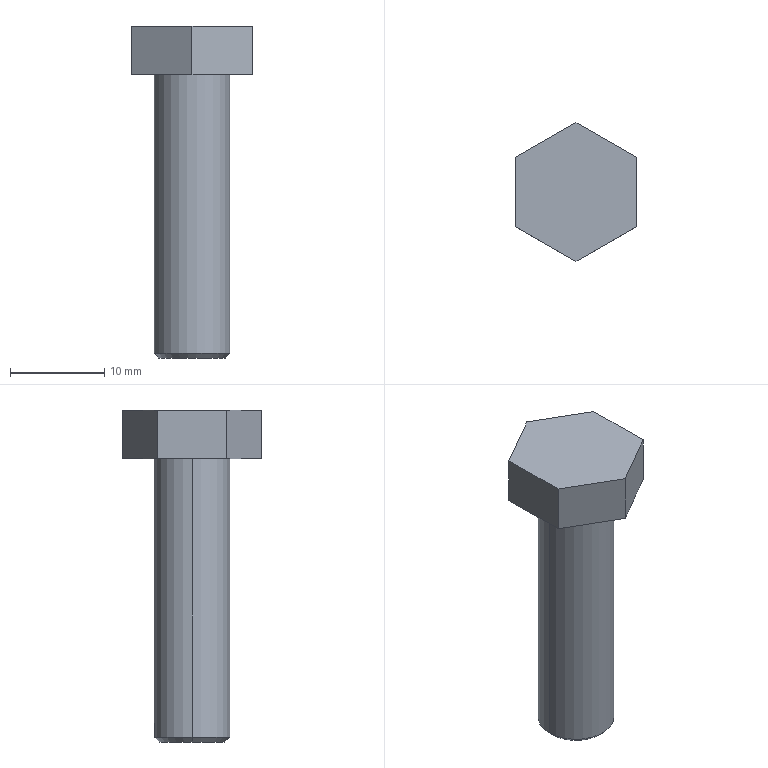Part | STEP file | Bulong M8_3F | 1 solid | 13 faces | box 12.73 x 14.699 x 35.15 mm | volume 2228 mm3 | plane 9 | cone 2 | cylinder 2 | commonest cylinder face diameters 8 x2
STEP:
#1=CARTESIAN_POINT('',(0.,0.,0.));
#2=DIRECTION('',(0.,0.,1.));
#3=DIRECTION('',(1.,0.,0.));
#4=AXIS2_PLACEMENT_3D('',#1,#2,#3);
#5=CARTESIAN_POINT('',(-3.5,0.,-30.));
#6=VERTEX_POINT('',#5);
#7=CARTESIAN_POINT('',(3.5,0.,-30.));
#8=VERTEX_POINT('',#7);
#9=CARTESIAN_POINT('',(0.,0.,-30.));
#10=DIRECTION('',(0.,0.,-1.));
#11=DIRECTION('',(-1.,0.,0.));
#12=AXIS2_PLACEMENT_3D('',#9,#10,#11);
#13=CIRCLE('',#12,3.5);
#14=CARTESIAN_POINT('',(0.,0.,-30.));
#15=DIRECTION('',(0.,0.,1.));
#16=DIRECTION('',(1.,0.,0.));
#17=AXIS2_PLACEMENT_3D('',#14,#15,#16);
#18=CONICAL_SURFACE('',#17,3.5,0.7854);
#19=CARTESIAN_POINT('',(3.142,0.));
#20=DIRECTION('',(-1.,0.));
#21=VECTOR('',#20,1.);
#22=LINE('',#19,#21);
#23=(GEOMETRIC_REPRESENTATION_CONTEXT(2)PARAMETRIC_REPRESENTATION_CONTEXT()REPRESENTATION_CONTEXT('',''));
#24=DEFINITIONAL_REPRESENTATION('',(#22),#23);
#25=PCURVE('',#18,#24);
#26=CARTESIAN_POINT('',(0.,0.,-30.));
#27=DIRECTION('',(0.,0.,-1.));
#28=DIRECTION('',(-1.,0.,0.));
#29=AXIS2_PLACEMENT_3D('',#26,#27,#28);
#30=PLANE('',#29);
#31=CARTESIAN_POINT('',(0.,0.));
#32=DIRECTION('',(1.,0.));
#33=AXIS2_PLACEMENT_2D('',#31,#32);
#34=CIRCLE('',#33,3.5);
#35=(GEOMETRIC_REPRESENTATION_CONTEXT(2)PARAMETRIC_REPRESENTATION_CONTEXT()REPRESENTATION_CONTEXT('',''));
#36=DEFINITIONAL_REPRESENTATION('',(#34),#35);
#37=PCURVE('',#30,#36);
#38=SURFACE_CURVE('',#13,(#25,#37),.PCURVE_S1.);
#39=EDGE_CURVE('',#6,#8,#38,.T.);
#40=ORIENTED_EDGE('',*,*,#39,.F.);
#41=CARTESIAN_POINT('',(-4.,0.,-29.5));
#42=VERTEX_POINT('',#41);
#43=CARTESIAN_POINT('',(-3.5,0.,-30.));
#44=DIRECTION('',(-0.7071,0.,0.7071));
#45=VECTOR('',#44,1.);
#46=LINE('',#43,#45);
#47=CARTESIAN_POINT('',(3.142,0.));
#48=DIRECTION('',(0.,1.));
#49=VECTOR('',#48,1.);
#50=LINE('',#47,#49);
#51=(GEOMETRIC_REPRESENTATION_CONTEXT(2)PARAMETRIC_REPRESENTATION_CONTEXT()REPRESENTATION_CONTEXT('',''));
#52=DEFINITIONAL_REPRESENTATION('',(#50),#51);
#53=PCURVE('',#18,#52);
#54=CARTESIAN_POINT('',(0.,0.,-30.));
#55=DIRECTION('',(0.,0.,1.));
#56=DIRECTION('',(1.,0.,0.));
#57=AXIS2_PLACEMENT_3D('',#54,#55,#56);
#58=CONICAL_SURFACE('',#57,3.5,0.7854);
#59=CARTESIAN_POINT('',(3.142,0.));
#60=DIRECTION('',(0.,1.));
#61=VECTOR('',#60,1.);
#62=LINE('',#59,#61);
#63=(GEOMETRIC_REPRESENTATION_CONTEXT(2)PARAMETRIC_REPRESENTATION_CONTEXT()REPRESENTATION_CONTEXT('',''));
#64=DEFINITIONAL_REPRESENTATION('',(#62),#63);
#65=PCURVE('',#58,#64);
#66=SURFACE_CURVE('',#46,(#53,#65),.PCURVE_S1.);
#67=EDGE_CURVE('',#6,#42,#66,.T.);
#68=ORIENTED_EDGE('',*,*,#67,.T.);
#69=CARTESIAN_POINT('',(4.,0.,-29.5));
#70=VERTEX_POINT('',#69);
#71=CARTESIAN_POINT('',(0.,0.,-29.5));
#72=DIRECTION('',(0.,0.,1.));
#73=DIRECTION('',(-1.,0.,0.));
#74=AXIS2_PLACEMENT_3D('',#71,#72,#73);
#75=CIRCLE('',#74,4.);
#76=CARTESIAN_POINT('',(-3.142,0.5));
#77=DIRECTION('',(1.,0.));
#78=VECTOR('',#77,1.);
#79=LINE('',#76,#78);
#80=(GEOMETRIC_REPRESENTATION_CONTEXT(2)PARAMETRIC_REPRESENTATION_CONTEXT()REPRESENTATION_CONTEXT('',''));
#81=DEFINITIONAL_REPRESENTATION('',(#79),#80);
#82=PCURVE('',#18,#81);
#83=CARTESIAN_POINT('',(0.,0.,-30.));
#84=DIRECTION('',(0.,0.,1.));
#85=DIRECTION('',(1.,0.,0.));
#86=AXIS2_PLACEMENT_3D('',#83,#84,#85);
#87=CYLINDRICAL_SURFACE('',#86,4.);
#88=CARTESIAN_POINT('',(-3.142,0.5));
#89=DIRECTION('',(1.,0.));
#90=VECTOR('',#89,1.);
#91=LINE('',#88,#90);
#92=(GEOMETRIC_REPRESENTATION_CONTEXT(2)PARAMETRIC_REPRESENTATION_CONTEXT()REPRESENTATION_CONTEXT('',''));
#93=DEFINITIONAL_REPRESENTATION('',(#91),#92);
#94=PCURVE('',#87,#93);
#95=SURFACE_CURVE('',#75,(#82,#94),.PCURVE_S1.);
#96=EDGE_CURVE('',#70,#42,#95,.T.);
#97=ORIENTED_EDGE('',*,*,#96,.F.);
#98=CARTESIAN_POINT('',(3.5,0.,-30.));
#99=DIRECTION('',(0.7071,0.,0.7071));
#100=VECTOR('',#99,1.);
#101=LINE('',#98,#100);
#102=CARTESIAN_POINT('',(0.,0.));
#103=DIRECTION('',(0.,1.));
#104=VECTOR('',#103,1.);
#105=LINE('',#102,#104);
#106=(GEOMETRIC_REPRESENTATION_CONTEXT(2)PARAMETRIC_REPRESENTATION_CONTEXT()REPRESENTATION_CONTEXT('',''));
#107=DEFINITIONAL_REPRESENTATION('',(#105),#106);
#108=PCURVE('',#18,#107);
#109=CARTESIAN_POINT('',(6.283,0.));
#110=DIRECTION('',(0.,1.));
#111=VECTOR('',#110,1.);
#112=LINE('',#109,#111);
#113=(GEOMETRIC_REPRESENTATION_CONTEXT(2)PARAMETRIC_REPRESENTATION_CONTEXT()REPRESENTATION_CONTEXT('',''));
#114=DEFINITIONAL_REPRESENTATION('',(#112),#113);
#115=PCURVE('',#58,#114);
#116=SURFACE_CURVE('',#101,(#108,#115),.PCURVE_S1.);
#117=EDGE_CURVE('',#8,#70,#116,.T.);
#118=ORIENTED_EDGE('',*,*,#117,.F.);
#119=EDGE_LOOP('',(#40,#68,#97,#118));
#120=FACE_BOUND('',#119,.T.);
#121=ADVANCED_FACE('',(#120),#18,.T.);
#122=ORIENTED_EDGE('',*,*,#96,.T.);
#123=CARTESIAN_POINT('',(-4.,0.,0.));
#124=VERTEX_POINT('',#123);
#125=CARTESIAN_POINT('',(-4.,0.,-30.));
#126=DIRECTION('',(0.,0.,1.));
#127=VECTOR('',#126,1.);
#128=LINE('',#125,#127);
#129=CARTESIAN_POINT('',(3.142,0.));
#130=DIRECTION('',(0.,1.));
#131=VECTOR('',#130,1.);
#132=LINE('',#129,#131);
#133=(GEOMETRIC_REPRESENTATION_CONTEXT(2)PARAMETRIC_REPRESENTATION_CONTEXT()REPRESENTATION_CONTEXT('',''));
#134=DEFINITIONAL_REPRESENTATION('',(#132),#133);
#135=PCURVE('',#87,#134);
#136=CARTESIAN_POINT('',(0.,0.,-30.));
#137=DIRECTION('',(0.,0.,1.));
#138=DIRECTION('',(1.,0.,0.));
#139=AXIS2_PLACEMENT_3D('',#136,#137,#138);
#140=CYLINDRICAL_SURFACE('',#139,4.);
#141=CARTESIAN_POINT('',(3.142,0.));
#142=DIRECTION('',(0.,1.));
#143=VECTOR('',#142,1.);
#144=LINE('',#141,#143);
#145=(GEOMETRIC_REPRESENTATION_CONTEXT(2)PARAMETRIC_REPRESENTATION_CONTEXT()REPRESENTATION_CONTEXT('',''));
#146=DEFINITIONAL_REPRESENTATION('',(#144),#145);
#147=PCURVE('',#140,#146);
#148=SURFACE_CURVE('',#128,(#135,#147),.PCURVE_S1.);
#149=EDGE_CURVE('',#42,#124,#148,.T.);
#150=ORIENTED_EDGE('',*,*,#149,.T.);
#151=CARTESIAN_POINT('',(4.,0.,0.));
#152=VERTEX_POINT('',#151);
#153=CARTESIAN_POINT('',(0.,0.,0.));
#154=DIRECTION('',(0.,0.,-1.));
#155=DIRECTION('',(1.,0.,0.));
#156=AXIS2_PLACEMENT_3D('',#153,#154,#155);
#157=CIRCLE('',#156,4.);
#158=CARTESIAN_POINT('',(6.283,30.));
#159=DIRECTION('',(-1.,0.));
#160=VECTOR('',#159,1.);
#161=LINE('',#158,#160);
#162=(GEOMETRIC_REPRESENTATION_CONTEXT(2)PARAMETRIC_REPRESENTATION_CONTEXT()REPRESENTATION_CONTEXT('',''));
#163=DEFINITIONAL_REPRESENTATION('',(#161),#162);
#164=PCURVE('',#87,#163);
#165=CARTESIAN_POINT('',(0.,0.,0.));
#166=DIRECTION('',(0.,0.,1.));
#167=DIRECTION('',(1.,0.,0.));
#168=AXIS2_PLACEMENT_3D('',#165,#166,#167);
#169=PLANE('',#168);
#170=CARTESIAN_POINT('',(4.,0.));
#171=CARTESIAN_POINT('',(4.,-6.928));
#172=CARTESIAN_POINT('',(-2.,-3.464));
#173=CARTESIAN_POINT('',(-8.,0.));
#174=CARTESIAN_POINT('',(-2.,3.464));
#175=CARTESIAN_POINT('',(4.,6.928));
#176=CARTESIAN_POINT('',(4.,0.));
#177=(BOUNDED_CURVE()B_SPLINE_CURVE(2,(#170,#171,#172,#173,#174,#175,#176),.UNSPECIFIED.,.T.,.F.)B_SPLINE_CURVE_WITH_KNOTS((1,2,2,2,2,1),(-2.094,0.,2.094,4.189,6.283,8.378),.UNSPECIFIED.)CURVE()GEOMETRIC_REPRESENTATION_ITEM()RATIONAL_B_SPLINE_CURVE((1.,0.5,1.,0.5,1.,0.5,1.))REPRESENTATION_ITEM(''));
#178=(GEOMETRIC_REPRESENTATION_CONTEXT(2)PARAMETRIC_REPRESENTATION_CONTEXT()REPRESENTATION_CONTEXT('',''));
#179=DEFINITIONAL_REPRESENTATION('',(#177),#178);
#180=PCURVE('',#169,#179);
#181=SURFACE_CURVE('',#157,(#164,#180),.PCURVE_S1.);
#182=EDGE_CURVE('',#124,#152,#181,.T.);
#183=ORIENTED_EDGE('',*,*,#182,.T.);
#184=CARTESIAN_POINT('',(4.,0.,-30.));
#185=DIRECTION('',(0.,0.,1.));
#186=VECTOR('',#185,1.);
#187=LINE('',#184,#186);
#188=CARTESIAN_POINT('',(0.,0.));
#189=DIRECTION('',(0.,1.));
#190=VECTOR('',#189,1.);
#191=LINE('',#188,#190);
#192=(GEOMETRIC_REPRESENTATION_CONTEXT(2)PARAMETRIC_REPRESENTATION_CONTEXT()REPRESENTATION_CONTEXT('',''));
#193=DEFINITIONAL_REPRESENTATION('',(#191),#192);
#194=PCURVE('',#87,#193);
#195=CARTESIAN_POINT('',(6.283,0.));
#196=DIRECTION('',(0.,1.));
#197=VECTOR('',#196,1.);
#198=LINE('',#195,#197);
#199=(GEOMETRIC_REPRESENTATION_CONTEXT(2)PARAMETRIC_REPRESENTATION_CONTEXT()REPRESENTATION_CONTEXT('',''));
#200=DEFINITIONAL_REPRESENTATION('',(#198),#199);
#201=PCURVE('',#140,#200);
#202=SURFACE_CURVE('',#187,(#194,#201),.PCURVE_S1.);
#203=EDGE_CURVE('',#70,#152,#202,.T.);
#204=ORIENTED_EDGE('',*,*,#203,.F.);
#205=EDGE_LOOP('',(#122,#150,#183,#204));
#206=FACE_BOUND('',#205,.T.);
#207=ADVANCED_FACE('',(#206),#87,.T.);
#208=CARTESIAN_POINT('',(6.365,3.675,0.));
#209=VERTEX_POINT('',#208);
#210=CARTESIAN_POINT('',(0.,7.35,0.));
#211=VERTEX_POINT('',#210);
#212=CARTESIAN_POINT('',(6.365,3.675,0.));
#213=DIRECTION('',(-0.866,0.5,0.));
#214=VECTOR('',#213,1.);
#215=LINE('',#212,#214);
#216=CARTESIAN_POINT('',(6.365,3.675));
#217=DIRECTION('',(-0.866,0.5));
#218=VECTOR('',#217,1.);
#219=LINE('',#216,#218);
#220=(GEOMETRIC_REPRESENTATION_CONTEXT(2)PARAMETRIC_REPRESENTATION_CONTEXT()REPRESENTATION_CONTEXT('',''));
#221=DEFINITIONAL_REPRESENTATION('',(#219),#220);
#222=PCURVE('',#169,#221);
#223=CARTESIAN_POINT('',(6.365,3.675,5.15));
#224=DIRECTION('',(-0.5,-0.866,0.));
#225=DIRECTION('',(0.866,-0.5,0.));
#226=AXIS2_PLACEMENT_3D('',#223,#224,#225);
#227=PLANE('',#226);
#228=CARTESIAN_POINT('',(0.,-5.15));
#229=DIRECTION('',(-1.,0.));
#230=VECTOR('',#229,1.);
#231=LINE('',#228,#230);
#232=(GEOMETRIC_REPRESENTATION_CONTEXT(2)PARAMETRIC_REPRESENTATION_CONTEXT()REPRESENTATION_CONTEXT('',''));
#233=DEFINITIONAL_REPRESENTATION('',(#231),#232);
#234=PCURVE('',#227,#233);
#235=SURFACE_CURVE('',#215,(#222,#234),.PCURVE_S1.);
#236=EDGE_CURVE('',#209,#211,#235,.T.);
#237=ORIENTED_EDGE('',*,*,#236,.F.);
#238=CARTESIAN_POINT('',(6.365,-3.675,0.));
#239=VERTEX_POINT('',#238);
#240=CARTESIAN_POINT('',(6.365,-3.675,0.));
#241=DIRECTION('',(0.,1.,0.));
#242=VECTOR('',#241,1.);
#243=LINE('',#240,#242);
#244=CARTESIAN_POINT('',(6.365,-3.675));
#245=DIRECTION('',(0.,1.));
#246=VECTOR('',#245,1.);
#247=LINE('',#244,#246);
#248=(GEOMETRIC_REPRESENTATION_CONTEXT(2)PARAMETRIC_REPRESENTATION_CONTEXT()REPRESENTATION_CONTEXT('',''));
#249=DEFINITIONAL_REPRESENTATION('',(#247),#248);
#250=PCURVE('',#169,#249);
#251=CARTESIAN_POINT('',(6.365,-3.675,5.15));
#252=DIRECTION('',(-1.,0.,0.));
#253=DIRECTION('',(0.,-1.,0.));
#254=AXIS2_PLACEMENT_3D('',#251,#252,#253);
#255=PLANE('',#254);
#256=CARTESIAN_POINT('',(0.,-5.15));
#257=DIRECTION('',(-1.,0.));
#258=VECTOR('',#257,1.);
#259=LINE('',#256,#258);
#260=(GEOMETRIC_REPRESENTATION_CONTEXT(2)PARAMETRIC_REPRESENTATION_CONTEXT()REPRESENTATION_CONTEXT('',''));
#261=DEFINITIONAL_REPRESENTATION('',(#259),#260);
#262=PCURVE('',#255,#261);
#263=SURFACE_CURVE('',#243,(#250,#262),.PCURVE_S1.);
#264=EDGE_CURVE('',#239,#209,#263,.T.);
#265=ORIENTED_EDGE('',*,*,#264,.F.);
#266=CARTESIAN_POINT('',(0.,-7.35,0.));
#267=VERTEX_POINT('',#266);
#268=CARTESIAN_POINT('',(0.,-7.35,0.));
#269=DIRECTION('',(0.866,0.5,0.));
#270=VECTOR('',#269,1.);
#271=LINE('',#268,#270);
#272=CARTESIAN_POINT('',(0.,-7.35));
#273=DIRECTION('',(0.866,0.5));
#274=VECTOR('',#273,1.);
#275=LINE('',#272,#274);
#276=(GEOMETRIC_REPRESENTATION_CONTEXT(2)PARAMETRIC_REPRESENTATION_CONTEXT()REPRESENTATION_CONTEXT('',''));
#277=DEFINITIONAL_REPRESENTATION('',(#275),#276);
#278=PCURVE('',#169,#277);
#279=CARTESIAN_POINT('',(0.,-7.35,5.15));
#280=DIRECTION('',(-0.5,0.866,0.));
#281=DIRECTION('',(-0.866,-0.5,0.));
#282=AXIS2_PLACEMENT_3D('',#279,#280,#281);
#283=PLANE('',#282);
#284=CARTESIAN_POINT('',(0.,-5.15));
#285=DIRECTION('',(-1.,0.));
#286=VECTOR('',#285,1.);
#287=LINE('',#284,#286);
#288=(GEOMETRIC_REPRESENTATION_CONTEXT(2)PARAMETRIC_REPRESENTATION_CONTEXT()REPRESENTATION_CONTEXT('',''));
#289=DEFINITIONAL_REPRESENTATION('',(#287),#288);
#290=PCURVE('',#283,#289);
#291=SURFACE_CURVE('',#271,(#278,#290),.PCURVE_S1.);
#292=EDGE_CURVE('',#267,#239,#291,.T.);
#293=ORIENTED_EDGE('',*,*,#292,.F.);
#294=CARTESIAN_POINT('',(-6.365,-3.675,0.));
#295=VERTEX_POINT('',#294);
#296=CARTESIAN_POINT('',(-6.365,-3.675,0.));
#297=DIRECTION('',(0.866,-0.5,0.));
#298=VECTOR('',#297,1.);
#299=LINE('',#296,#298);
#300=CARTESIAN_POINT('',(-6.365,-3.675));
#301=DIRECTION('',(0.866,-0.5));
#302=VECTOR('',#301,1.);
#303=LINE('',#300,#302);
#304=(GEOMETRIC_REPRESENTATION_CONTEXT(2)PARAMETRIC_REPRESENTATION_CONTEXT()REPRESENTATION_CONTEXT('',''));
#305=DEFINITIONAL_REPRESENTATION('',(#303),#304);
#306=PCURVE('',#169,#305);
#307=CARTESIAN_POINT('',(-6.365,-3.675,5.15));
#308=DIRECTION('',(0.5,0.866,0.));
#309=DIRECTION('',(-0.866,0.5,0.));
#310=AXIS2_PLACEMENT_3D('',#307,#308,#309);
#311=PLANE('',#310);
#312=CARTESIAN_POINT('',(0.,-5.15));
#313=DIRECTION('',(-1.,0.));
#314=VECTOR('',#313,1.);
#315=LINE('',#312,#314);
#316=(GEOMETRIC_REPRESENTATION_CONTEXT(2)PARAMETRIC_REPRESENTATION_CONTEXT()REPRESENTATION_CONTEXT('',''));
#317=DEFINITIONAL_REPRESENTATION('',(#315),#316);
#318=PCURVE('',#311,#317);
#319=SURFACE_CURVE('',#299,(#306,#318),.PCURVE_S1.);
#320=EDGE_CURVE('',#295,#267,#319,.T.);
#321=ORIENTED_EDGE('',*,*,#320,.F.);
#322=CARTESIAN_POINT('',(-6.365,3.675,0.));
#323=VERTEX_POINT('',#322);
#324=CARTESIAN_POINT('',(-6.365,3.675,0.));
#325=DIRECTION('',(0.,-1.,0.));
#326=VECTOR('',#325,1.);
#327=LINE('',#324,#326);
#328=CARTESIAN_POINT('',(-6.365,3.675));
#329=DIRECTION('',(0.,-1.));
#330=VECTOR('',#329,1.);
#331=LINE('',#328,#330);
#332=(GEOMETRIC_REPRESENTATION_CONTEXT(2)PARAMETRIC_REPRESENTATION_CONTEXT()REPRESENTATION_CONTEXT('',''));
#333=DEFINITIONAL_REPRESENTATION('',(#331),#332);
#334=PCURVE('',#169,#333);
#335=CARTESIAN_POINT('',(-6.365,3.675,5.15));
#336=DIRECTION('',(1.,0.,0.));
#337=DIRECTION('',(0.,0.,-1.));
#338=AXIS2_PLACEMENT_3D('',#335,#336,#337);
#339=PLANE('',#338);
#340=CARTESIAN_POINT('',(5.15,0.));
#341=DIRECTION('',(0.,-1.));
#342=VECTOR('',#341,1.);
#343=LINE('',#340,#342);
#344=(GEOMETRIC_REPRESENTATION_CONTEXT(2)PARAMETRIC_REPRESENTATION_CONTEXT()REPRESENTATION_CONTEXT('',''));
#345=DEFINITIONAL_REPRESENTATION('',(#343),#344);
#346=PCURVE('',#339,#345);
#347=SURFACE_CURVE('',#327,(#334,#346),.PCURVE_S1.);
#348=EDGE_CURVE('',#323,#295,#347,.T.);
#349=ORIENTED_EDGE('',*,*,#348,.F.);
#350=CARTESIAN_POINT('',(0.,7.35,0.));
#351=DIRECTION('',(-0.866,-0.5,0.));
#352=VECTOR('',#351,1.);
#353=LINE('',#350,#352);
#354=CARTESIAN_POINT('',(0.,7.35));
#355=DIRECTION('',(-0.866,-0.5));
#356=VECTOR('',#355,1.);
#357=LINE('',#354,#356);
#358=(GEOMETRIC_REPRESENTATION_CONTEXT(2)PARAMETRIC_REPRESENTATION_CONTEXT()REPRESENTATION_CONTEXT('',''));
#359=DEFINITIONAL_REPRESENTATION('',(#357),#358);
#360=PCURVE('',#169,#359);
#361=CARTESIAN_POINT('',(0.,7.35,5.15));
#362=DIRECTION('',(0.5,-0.866,0.));
#363=DIRECTION('',(0.866,0.5,0.));
#364=AXIS2_PLACEMENT_3D('',#361,#362,#363);
#365=PLANE('',#364);
#366=CARTESIAN_POINT('',(0.,-5.15));
#367=DIRECTION('',(-1.,0.));
#368=VECTOR('',#367,1.);
#369=LINE('',#366,#368);
#370=(GEOMETRIC_REPRESENTATION_CONTEXT(2)PARAMETRIC_REPRESENTATION_CONTEXT()REPRESENTATION_CONTEXT('',''));
#371=DEFINITIONAL_REPRESENTATION('',(#369),#370);
#372=PCURVE('',#365,#371);
#373=SURFACE_CURVE('',#353,(#360,#372),.PCURVE_S1.);
#374=EDGE_CURVE('',#211,#323,#373,.T.);
#375=ORIENTED_EDGE('',*,*,#374,.F.);
#376=EDGE_LOOP('',(#237,#265,#293,#321,#349,#375));
#377=FACE_BOUND('',#376,.T.);
#378=CARTESIAN_POINT('',(0.,0.,0.));
#379=DIRECTION('',(0.,0.,-1.));
#380=DIRECTION('',(1.,0.,0.));
#381=AXIS2_PLACEMENT_3D('',#378,#379,#380);
#382=CIRCLE('',#381,4.);
#383=CARTESIAN_POINT('',(4.,0.));
#384=CARTESIAN_POINT('',(4.,-6.928));
#385=CARTESIAN_POINT('',(-2.,-3.464));
#386=CARTESIAN_POINT('',(-8.,0.));
#387=CARTESIAN_POINT('',(-2.,3.464));
#388=CARTESIAN_POINT('',(4.,6.928));
#389=CARTESIAN_POINT('',(4.,0.));
#390=(BOUNDED_CURVE()B_SPLINE_CURVE(2,(#383,#384,#385,#386,#387,#388,#389),.UNSPECIFIED.,.T.,.F.)B_SPLINE_CURVE_WITH_KNOTS((1,2,2,2,2,1),(-2.094,0.,2.094,4.189,6.283,8.378),.UNSPECIFIED.)CURVE()GEOMETRIC_REPRESENTATION_ITEM()RATIONAL_B_SPLINE_CURVE((1.,0.5,1.,0.5,1.,0.5,1.))REPRESENTATION_ITEM(''));
#391=(GEOMETRIC_REPRESENTATION_CONTEXT(2)PARAMETRIC_REPRESENTATION_CONTEXT()REPRESENTATION_CONTEXT('',''));
#392=DEFINITIONAL_REPRESENTATION('',(#390),#391);
#393=PCURVE('',#169,#392);
#394=CARTESIAN_POINT('',(6.283,30.));
#395=DIRECTION('',(-1.,0.));
#396=VECTOR('',#395,1.);
#397=LINE('',#394,#396);
#398=(GEOMETRIC_REPRESENTATION_CONTEXT(2)PARAMETRIC_REPRESENTATION_CONTEXT()REPRESENTATION_CONTEXT('',''));
#399=DEFINITIONAL_REPRESENTATION('',(#397),#398);
#400=PCURVE('',#140,#399);
#401=SURFACE_CURVE('',#382,(#393,#400),.PCURVE_S1.);
#402=EDGE_CURVE('',#152,#124,#401,.T.);
#403=ORIENTED_EDGE('',*,*,#402,.F.);
#404=ORIENTED_EDGE('',*,*,#182,.F.);
#405=EDGE_LOOP('',(#403,#404));
#406=FACE_BOUND('',#405,.T.);
#407=ADVANCED_FACE('',(#377,#406),#169,.F.);
#408=ORIENTED_EDGE('',*,*,#236,.T.);
#409=CARTESIAN_POINT('',(0.,7.35,5.15));
#410=VERTEX_POINT('',#409);
#411=CARTESIAN_POINT('',(0.,7.35,5.15));
#412=DIRECTION('',(0.,0.,-1.));
#413=VECTOR('',#412,1.);
#414=LINE('',#411,#413);
#415=CARTESIAN_POINT('',(-7.35,0.));
#416=DIRECTION('',(0.,-1.));
#417=VECTOR('',#416,1.);
#418=LINE('',#415,#417);
#419=(GEOMETRIC_REPRESENTATION_CONTEXT(2)PARAMETRIC_REPRESENTATION_CONTEXT()REPRESENTATION_CONTEXT('',''));
#420=DEFINITIONAL_REPRESENTATION('',(#418),#419);
#421=PCURVE('',#227,#420);
#422=CARTESIAN_POINT('',(0.,0.));
#423=DIRECTION('',(0.,-1.));
#424=VECTOR('',#423,1.);
#425=LINE('',#422,#424);
#426=(GEOMETRIC_REPRESENTATION_CONTEXT(2)PARAMETRIC_REPRESENTATION_CONTEXT()REPRESENTATION_CONTEXT('',''));
#427=DEFINITIONAL_REPRESENTATION('',(#425),#426);
#428=PCURVE('',#365,#427);
#429=SURFACE_CURVE('',#414,(#421,#428),.PCURVE_S1.);
#430=EDGE_CURVE('',#410,#211,#429,.T.);
#431=ORIENTED_EDGE('',*,*,#430,.F.);
#432=CARTESIAN_POINT('',(6.365,3.675,5.15));
#433=VERTEX_POINT('',#432);
#434=CARTESIAN_POINT('',(6.365,3.675,5.15));
#435=DIRECTION('',(-0.866,0.5,0.));
#436=VECTOR('',#435,1.);
#437=LINE('',#434,#436);
#438=CARTESIAN_POINT('',(0.,0.));
#439=DIRECTION('',(-1.,0.));
#440=VECTOR('',#439,1.);
#441=LINE('',#438,#440);
#442=(GEOMETRIC_REPRESENTATION_CONTEXT(2)PARAMETRIC_REPRESENTATION_CONTEXT()REPRESENTATION_CONTEXT('',''));
#443=DEFINITIONAL_REPRESENTATION('',(#441),#442);
#444=PCURVE('',#227,#443);
#445=CARTESIAN_POINT('',(0.,0.,5.15));
#446=DIRECTION('',(0.,0.,1.));
#447=DIRECTION('',(1.,0.,0.));
#448=AXIS2_PLACEMENT_3D('',#445,#446,#447);
#449=PLANE('',#448);
#450=CARTESIAN_POINT('',(6.365,3.675));
#451=DIRECTION('',(-0.866,0.5));
#452=VECTOR('',#451,1.);
#453=LINE('',#450,#452);
#454=(GEOMETRIC_REPRESENTATION_CONTEXT(2)PARAMETRIC_REPRESENTATION_CONTEXT()REPRESENTATION_CONTEXT('',''));
#455=DEFINITIONAL_REPRESENTATION('',(#453),#454);
#456=PCURVE('',#449,#455);
#457=SURFACE_CURVE('',#437,(#444,#456),.PCURVE_S1.);
#458=EDGE_CURVE('',#433,#410,#457,.T.);
#459=ORIENTED_EDGE('',*,*,#458,.F.);
#460=CARTESIAN_POINT('',(6.365,3.675,5.15));
#461=DIRECTION('',(0.,0.,-1.));
#462=VECTOR('',#461,1.);
#463=LINE('',#460,#462);
#464=CARTESIAN_POINT('',(0.,0.));
#465=DIRECTION('',(0.,-1.));
#466=VECTOR('',#465,1.);
#467=LINE('',#464,#466);
#468=(GEOMETRIC_REPRESENTATION_CONTEXT(2)PARAMETRIC_REPRESENTATION_CONTEXT()REPRESENTATION_CONTEXT('',''));
#469=DEFINITIONAL_REPRESENTATION('',(#467),#468);
#470=PCURVE('',#227,#469);
#471=CARTESIAN_POINT('',(-7.35,0.));
#472=DIRECTION('',(0.,-1.));
#473=VECTOR('',#472,1.);
#474=LINE('',#471,#473);
#475=(GEOMETRIC_REPRESENTATION_CONTEXT(2)PARAMETRIC_REPRESENTATION_CONTEXT()REPRESENTATION_CONTEXT('',''));
#476=DEFINITIONAL_REPRESENTATION('',(#474),#475);
#477=PCURVE('',#255,#476);
#478=SURFACE_CURVE('',#463,(#470,#477),.PCURVE_S1.);
#479=EDGE_CURVE('',#433,#209,#478,.T.);
#480=ORIENTED_EDGE('',*,*,#479,.T.);
#481=EDGE_LOOP('',(#408,#431,#459,#480));
#482=FACE_BOUND('',#481,.T.);
#483=ADVANCED_FACE('',(#482),#227,.F.);
#484=ORIENTED_EDGE('',*,*,#374,.T.);
#485=CARTESIAN_POINT('',(-6.365,3.675,5.15));
#486=VERTEX_POINT('',#485);
#487=CARTESIAN_POINT('',(-6.365,3.675,5.15));
#488=DIRECTION('',(0.,0.,-1.));
#489=VECTOR('',#488,1.);
#490=LINE('',#487,#489);
#491=CARTESIAN_POINT('',(-7.35,0.));
#492=DIRECTION('',(0.,-1.));
#493=VECTOR('',#492,1.);
#494=LINE('',#491,#493);
#495=(GEOMETRIC_REPRESENTATION_CONTEXT(2)PARAMETRIC_REPRESENTATION_CONTEXT()REPRESENTATION_CONTEXT('',''));
#496=DEFINITIONAL_REPRESENTATION('',(#494),#495);
#497=PCURVE('',#365,#496);
#498=CARTESIAN_POINT('',(0.,0.));
#499=DIRECTION('',(1.,0.));
#500=VECTOR('',#499,1.);
#501=LINE('',#498,#500);
#502=(GEOMETRIC_REPRESENTATION_CONTEXT(2)PARAMETRIC_REPRESENTATION_CONTEXT()REPRESENTATION_CONTEXT('',''));
#503=DEFINITIONAL_REPRESENTATION('',(#501),#502);
#504=PCURVE('',#339,#503);
#505=SURFACE_CURVE('',#490,(#497,#504),.PCURVE_S1.);
#506=EDGE_CURVE('',#486,#323,#505,.T.);
#507=ORIENTED_EDGE('',*,*,#506,.F.);
#508=CARTESIAN_POINT('',(0.,7.35,5.15));
#509=DIRECTION('',(-0.866,-0.5,0.));
#510=VECTOR('',#509,1.);
#511=LINE('',#508,#510);
#512=CARTESIAN_POINT('',(0.,0.));
#513=DIRECTION('',(-1.,0.));
#514=VECTOR('',#513,1.);
#515=LINE('',#512,#514);
#516=(GEOMETRIC_REPRESENTATION_CONTEXT(2)PARAMETRIC_REPRESENTATION_CONTEXT()REPRESENTATION_CONTEXT('',''));
#517=DEFINITIONAL_REPRESENTATION('',(#515),#516);
#518=PCURVE('',#365,#517);
#519=CARTESIAN_POINT('',(0.,7.35));
#520=DIRECTION('',(-0.866,-0.5));
#521=VECTOR('',#520,1.);
#522=LINE('',#519,#521);
#523=(GEOMETRIC_REPRESENTATION_CONTEXT(2)PARAMETRIC_REPRESENTATION_CONTEXT()REPRESENTATION_CONTEXT('',''));
#524=DEFINITIONAL_REPRESENTATION('',(#522),#523);
#525=PCURVE('',#449,#524);
#526=SURFACE_CURVE('',#511,(#518,#525),.PCURVE_S1.);
#527=EDGE_CURVE('',#410,#486,#526,.T.);
#528=ORIENTED_EDGE('',*,*,#527,.F.);
#529=ORIENTED_EDGE('',*,*,#430,.T.);
#530=EDGE_LOOP('',(#484,#507,#528,#529));
#531=FACE_BOUND('',#530,.T.);
#532=ADVANCED_FACE('',(#531),#365,.F.);
#533=ORIENTED_EDGE('',*,*,#348,.T.);
#534=CARTESIAN_POINT('',(-6.365,-3.675,5.15));
#535=VERTEX_POINT('',#534);
#536=CARTESIAN_POINT('',(-6.365,-3.675,5.15));
#537=DIRECTION('',(0.,0.,-1.));
#538=VECTOR('',#537,1.);
#539=LINE('',#536,#538);
#540=CARTESIAN_POINT('',(0.,-7.35));
#541=DIRECTION('',(1.,0.));
#542=VECTOR('',#541,1.);
#543=LINE('',#540,#542);
#544=(GEOMETRIC_REPRESENTATION_CONTEXT(2)PARAMETRIC_REPRESENTATION_CONTEXT()REPRESENTATION_CONTEXT('',''));
#545=DEFINITIONAL_REPRESENTATION('',(#543),#544);
#546=PCURVE('',#339,#545);
#547=CARTESIAN_POINT('',(0.,0.));
#548=DIRECTION('',(0.,-1.));
#549=VECTOR('',#548,1.);
#550=LINE('',#547,#549);
#551=(GEOMETRIC_REPRESENTATION_CONTEXT(2)PARAMETRIC_REPRESENTATION_CONTEXT()REPRESENTATION_CONTEXT('',''));
#552=DEFINITIONAL_REPRESENTATION('',(#550),#551);
#553=PCURVE('',#311,#552);
#554=SURFACE_CURVE('',#539,(#546,#553),.PCURVE_S1.);
#555=EDGE_CURVE('',#535,#295,#554,.T.);
#556=ORIENTED_EDGE('',*,*,#555,.F.);
#557=CARTESIAN_POINT('',(-6.365,3.675,5.15));
#558=DIRECTION('',(0.,-1.,0.));
#559=VECTOR('',#558,1.);
#560=LINE('',#557,#559);
#561=CARTESIAN_POINT('',(0.,0.));
#562=DIRECTION('',(0.,-1.));
#563=VECTOR('',#562,1.);
#564=LINE('',#561,#563);
#565=(GEOMETRIC_REPRESENTATION_CONTEXT(2)PARAMETRIC_REPRESENTATION_CONTEXT()REPRESENTATION_CONTEXT('',''));
#566=DEFINITIONAL_REPRESENTATION('',(#564),#565);
#567=PCURVE('',#339,#566);
#568=CARTESIAN_POINT('',(-6.365,3.675));
#569=DIRECTION('',(0.,-1.));
#570=VECTOR('',#569,1.);
#571=LINE('',#568,#570);
#572=(GEOMETRIC_REPRESENTATION_CONTEXT(2)PARAMETRIC_REPRESENTATION_CONTEXT()REPRESENTATION_CONTEXT('',''));
#573=DEFINITIONAL_REPRESENTATION('',(#571),#572);
#574=PCURVE('',#449,#573);
#575=SURFACE_CURVE('',#560,(#567,#574),.PCURVE_S1.);
#576=EDGE_CURVE('',#486,#535,#575,.T.);
#577=ORIENTED_EDGE('',*,*,#576,.F.);
#578=ORIENTED_EDGE('',*,*,#506,.T.);
#579=EDGE_LOOP('',(#533,#556,#577,#578));
#580=FACE_BOUND('',#579,.T.);
#581=ADVANCED_FACE('',(#580),#339,.F.);
#582=ORIENTED_EDGE('',*,*,#320,.T.);
#583=CARTESIAN_POINT('',(0.,-7.35,5.15));
#584=VERTEX_POINT('',#583);
#585=CARTESIAN_POINT('',(0.,-7.35,5.15));
#586=DIRECTION('',(0.,0.,-1.));
#587=VECTOR('',#586,1.);
#588=LINE('',#585,#587);
#589=CARTESIAN_POINT('',(-7.35,0.));
#590=DIRECTION('',(0.,-1.));
#591=VECTOR('',#590,1.);
#592=LINE('',#589,#591);
#593=(GEOMETRIC_REPRESENTATION_CONTEXT(2)PARAMETRIC_REPRESENTATION_CONTEXT()REPRESENTATION_CONTEXT('',''));
#594=DEFINITIONAL_REPRESENTATION('',(#592),#593);
#595=PCURVE('',#311,#594);
#596=CARTESIAN_POINT('',(0.,0.));
#597=DIRECTION('',(0.,-1.));
#598=VECTOR('',#597,1.);
#599=LINE('',#596,#598);
#600=(GEOMETRIC_REPRESENTATION_CONTEXT(2)PARAMETRIC_REPRESENTATION_CONTEXT()REPRESENTATION_CONTEXT('',''));
#601=DEFINITIONAL_REPRESENTATION('',(#599),#600);
#602=PCURVE('',#283,#601);
#603=SURFACE_CURVE('',#588,(#595,#602),.PCURVE_S1.);
#604=EDGE_CURVE('',#584,#267,#603,.T.);
#605=ORIENTED_EDGE('',*,*,#604,.F.);
#606=CARTESIAN_POINT('',(-6.365,-3.675,5.15));
#607=DIRECTION('',(0.866,-0.5,0.));
#608=VECTOR('',#607,1.);
#609=LINE('',#606,#608);
#610=CARTESIAN_POINT('',(0.,0.));
#611=DIRECTION('',(-1.,0.));
#612=VECTOR('',#611,1.);
#613=LINE('',#610,#612);
#614=(GEOMETRIC_REPRESENTATION_CONTEXT(2)PARAMETRIC_REPRESENTATION_CONTEXT()REPRESENTATION_CONTEXT('',''));
#615=DEFINITIONAL_REPRESENTATION('',(#613),#614);
#616=PCURVE('',#311,#615);
#617=CARTESIAN_POINT('',(-6.365,-3.675));
#618=DIRECTION('',(0.866,-0.5));
#619=VECTOR('',#618,1.);
#620=LINE('',#617,#619);
#621=(GEOMETRIC_REPRESENTATION_CONTEXT(2)PARAMETRIC_REPRESENTATION_CONTEXT()REPRESENTATION_CONTEXT('',''));
#622=DEFINITIONAL_REPRESENTATION('',(#620),#621);
#623=PCURVE('',#449,#622);
#624=SURFACE_CURVE('',#609,(#616,#623),.PCURVE_S1.);
#625=EDGE_CURVE('',#535,#584,#624,.T.);
#626=ORIENTED_EDGE('',*,*,#625,.F.);
#627=ORIENTED_EDGE('',*,*,#555,.T.);
#628=EDGE_LOOP('',(#582,#605,#626,#627));
#629=FACE_BOUND('',#628,.T.);
#630=ADVANCED_FACE('',(#629),#311,.F.);
#631=ORIENTED_EDGE('',*,*,#292,.T.);
#632=CARTESIAN_POINT('',(6.365,-3.675,5.15));
#633=VERTEX_POINT('',#632);
#634=CARTESIAN_POINT('',(6.365,-3.675,5.15));
#635=DIRECTION('',(0.,0.,-1.));
#636=VECTOR('',#635,1.);
#637=LINE('',#634,#636);
#638=CARTESIAN_POINT('',(-7.35,0.));
#639=DIRECTION('',(0.,-1.));
#640=VECTOR('',#639,1.);
#641=LINE('',#638,#640);
#642=(GEOMETRIC_REPRESENTATION_CONTEXT(2)PARAMETRIC_REPRESENTATION_CONTEXT()REPRESENTATION_CONTEXT('',''));
#643=DEFINITIONAL_REPRESENTATION('',(#641),#642);
#644=PCURVE('',#283,#643);
#645=CARTESIAN_POINT('',(0.,0.));
#646=DIRECTION('',(0.,-1.));
#647=VECTOR('',#646,1.);
#648=LINE('',#645,#647);
#649=(GEOMETRIC_REPRESENTATION_CONTEXT(2)PARAMETRIC_REPRESENTATION_CONTEXT()REPRESENTATION_CONTEXT('',''));
#650=DEFINITIONAL_REPRESENTATION('',(#648),#649);
#651=PCURVE('',#255,#650);
#652=SURFACE_CURVE('',#637,(#644,#651),.PCURVE_S1.);
#653=EDGE_CURVE('',#633,#239,#652,.T.);
#654=ORIENTED_EDGE('',*,*,#653,.F.);
#655=CARTESIAN_POINT('',(0.,-7.35,5.15));
#656=DIRECTION('',(0.866,0.5,0.));
#657=VECTOR('',#656,1.);
#658=LINE('',#655,#657);
#659=CARTESIAN_POINT('',(0.,0.));
#660=DIRECTION('',(-1.,0.));
#661=VECTOR('',#660,1.);
#662=LINE('',#659,#661);
#663=(GEOMETRIC_REPRESENTATION_CONTEXT(2)PARAMETRIC_REPRESENTATION_CONTEXT()REPRESENTATION_CONTEXT('',''));
#664=DEFINITIONAL_REPRESENTATION('',(#662),#663);
#665=PCURVE('',#283,#664);
#666=CARTESIAN_POINT('',(0.,-7.35));
#667=DIRECTION('',(0.866,0.5));
#668=VECTOR('',#667,1.);
#669=LINE('',#666,#668);
#670=(GEOMETRIC_REPRESENTATION_CONTEXT(2)PARAMETRIC_REPRESENTATION_CONTEXT()REPRESENTATION_CONTEXT('',''));
#671=DEFINITIONAL_REPRESENTATION('',(#669),#670);
#672=PCURVE('',#449,#671);
#673=SURFACE_CURVE('',#658,(#665,#672),.PCURVE_S1.);
#674=EDGE_CURVE('',#584,#633,#673,.T.);
#675=ORIENTED_EDGE('',*,*,#674,.F.);
#676=ORIENTED_EDGE('',*,*,#604,.T.);
#677=EDGE_LOOP('',(#631,#654,#675,#676));
#678=FACE_BOUND('',#677,.T.);
#679=ADVANCED_FACE('',(#678),#283,.F.);
#680=ORIENTED_EDGE('',*,*,#264,.T.);
#681=ORIENTED_EDGE('',*,*,#479,.F.);
#682=CARTESIAN_POINT('',(6.365,-3.675,5.15));
#683=DIRECTION('',(0.,1.,0.));
#684=VECTOR('',#683,1.);
#685=LINE('',#682,#684);
#686=CARTESIAN_POINT('',(0.,0.));
#687=DIRECTION('',(-1.,0.));
#688=VECTOR('',#687,1.);
#689=LINE('',#686,#688);
#690=(GEOMETRIC_REPRESENTATION_CONTEXT(2)PARAMETRIC_REPRESENTATION_CONTEXT()REPRESENTATION_CONTEXT('',''));
#691=DEFINITIONAL_REPRESENTATION('',(#689),#690);
#692=PCURVE('',#255,#691);
#693=CARTESIAN_POINT('',(6.365,-3.675));
#694=DIRECTION('',(0.,1.));
#695=VECTOR('',#694,1.);
#696=LINE('',#693,#695);
#697=(GEOMETRIC_REPRESENTATION_CONTEXT(2)PARAMETRIC_REPRESENTATION_CONTEXT()REPRESENTATION_CONTEXT('',''));
#698=DEFINITIONAL_REPRESENTATION('',(#696),#697);
#699=PCURVE('',#449,#698);
#700=SURFACE_CURVE('',#685,(#692,#699),.PCURVE_S1.);
#701=EDGE_CURVE('',#633,#433,#700,.T.);
#702=ORIENTED_EDGE('',*,*,#701,.F.);
#703=ORIENTED_EDGE('',*,*,#653,.T.);
#704=EDGE_LOOP('',(#680,#681,#702,#703));
#705=FACE_BOUND('',#704,.T.);
#706=ADVANCED_FACE('',(#705),#255,.F.);
#707=ORIENTED_EDGE('',*,*,#458,.T.);
#708=ORIENTED_EDGE('',*,*,#527,.T.);
#709=ORIENTED_EDGE('',*,*,#576,.T.);
#710=ORIENTED_EDGE('',*,*,#625,.T.);
#711=ORIENTED_EDGE('',*,*,#674,.T.);
#712=ORIENTED_EDGE('',*,*,#701,.T.);
#713=EDGE_LOOP('',(#707,#708,#709,#710,#711,#712));
#714=FACE_BOUND('',#713,.T.);
#715=ADVANCED_FACE('',(#714),#449,.T.);
#716=ORIENTED_EDGE('',*,*,#149,.F.);
#717=CARTESIAN_POINT('',(0.,0.,-29.5));
#718=DIRECTION('',(0.,0.,1.));
#719=DIRECTION('',(-1.,0.,0.));
#720=AXIS2_PLACEMENT_3D('',#717,#718,#719);
#721=CIRCLE('',#720,4.);
#722=CARTESIAN_POINT('',(3.142,0.5));
#723=DIRECTION('',(1.,0.));
#724=VECTOR('',#723,1.);
#725=LINE('',#722,#724);
#726=(GEOMETRIC_REPRESENTATION_CONTEXT(2)PARAMETRIC_REPRESENTATION_CONTEXT()REPRESENTATION_CONTEXT('',''));
#727=DEFINITIONAL_REPRESENTATION('',(#725),#726);
#728=PCURVE('',#140,#727);
#729=CARTESIAN_POINT('',(3.142,0.5));
#730=DIRECTION('',(1.,0.));
#731=VECTOR('',#730,1.);
#732=LINE('',#729,#731);
#733=(GEOMETRIC_REPRESENTATION_CONTEXT(2)PARAMETRIC_REPRESENTATION_CONTEXT()REPRESENTATION_CONTEXT('',''));
#734=DEFINITIONAL_REPRESENTATION('',(#732),#733);
#735=PCURVE('',#58,#734);
#736=SURFACE_CURVE('',#721,(#728,#735),.PCURVE_S1.);
#737=EDGE_CURVE('',#42,#70,#736,.T.);
#738=ORIENTED_EDGE('',*,*,#737,.T.);
#739=ORIENTED_EDGE('',*,*,#203,.T.);
#740=ORIENTED_EDGE('',*,*,#402,.T.);
#741=EDGE_LOOP('',(#716,#738,#739,#740));
#742=FACE_BOUND('',#741,.T.);
#743=ADVANCED_FACE('',(#742),#140,.T.);
#744=CARTESIAN_POINT('',(0.,0.,-30.));
#745=DIRECTION('',(0.,0.,-1.));
#746=DIRECTION('',(-1.,0.,0.));
#747=AXIS2_PLACEMENT_3D('',#744,#745,#746);
#748=CIRCLE('',#747,3.5);
#749=CARTESIAN_POINT('',(0.,0.));
#750=DIRECTION('',(1.,0.));
#751=AXIS2_PLACEMENT_2D('',#749,#750);
#752=CIRCLE('',#751,3.5);
#753=(GEOMETRIC_REPRESENTATION_CONTEXT(2)PARAMETRIC_REPRESENTATION_CONTEXT()REPRESENTATION_CONTEXT('',''));
#754=DEFINITIONAL_REPRESENTATION('',(#752),#753);
#755=PCURVE('',#30,#754);
#756=CARTESIAN_POINT('',(9.425,0.));
#757=DIRECTION('',(-1.,0.));
#758=VECTOR('',#757,1.);
#759=LINE('',#756,#758);
#760=(GEOMETRIC_REPRESENTATION_CONTEXT(2)PARAMETRIC_REPRESENTATION_CONTEXT()REPRESENTATION_CONTEXT('',''));
#761=DEFINITIONAL_REPRESENTATION('',(#759),#760);
#762=PCURVE('',#58,#761);
#763=SURFACE_CURVE('',#748,(#755,#762),.PCURVE_S1.);
#764=EDGE_CURVE('',#8,#6,#763,.T.);
#765=ORIENTED_EDGE('',*,*,#764,.T.);
#766=ORIENTED_EDGE('',*,*,#39,.T.);
#767=EDGE_LOOP('',(#765,#766));
#768=FACE_BOUND('',#767,.T.);
#769=ADVANCED_FACE('',(#768),#30,.T.);
#770=ORIENTED_EDGE('',*,*,#67,.F.);
#771=ORIENTED_EDGE('',*,*,#764,.F.);
#772=ORIENTED_EDGE('',*,*,#117,.T.);
#773=ORIENTED_EDGE('',*,*,#737,.F.);
#774=EDGE_LOOP('',(#770,#771,#772,#773));
#775=FACE_BOUND('',#774,.T.);
#776=ADVANCED_FACE('',(#775),#58,.T.);
#777=CLOSED_SHELL('',(#121,#207,#407,#483,#532,#581,#630,#679,#706,#715,#743,#769,#776));
#778=MANIFOLD_SOLID_BREP('',#777);
#779=(LENGTH_UNIT()NAMED_UNIT(*)SI_UNIT(.MILLI.,.METRE.));
#780=UNCERTAINTY_MEASURE_WITH_UNIT(LENGTH_MEASURE(0.0000001),#779,'','');
#781=(NAMED_UNIT(*)PLANE_ANGLE_UNIT()SI_UNIT($,.RADIAN.));
#782=(NAMED_UNIT(*)SI_UNIT($,.STERADIAN.)SOLID_ANGLE_UNIT());
#783=(GEOMETRIC_REPRESENTATION_CONTEXT(3)GLOBAL_UNCERTAINTY_ASSIGNED_CONTEXT((#780))GLOBAL_UNIT_ASSIGNED_CONTEXT((#779,#781,#782))REPRESENTATION_CONTEXT('',''));
#784=ADVANCED_BREP_SHAPE_REPRESENTATION('',(#4,#778),#783);